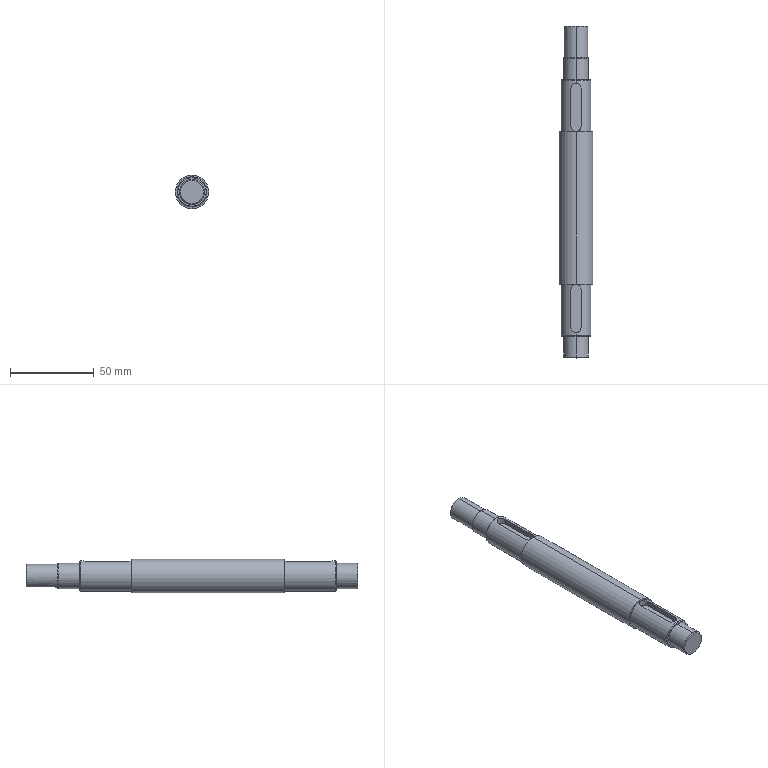Part | STEP file | 1 solid | 42 faces | box 20 x 198 x 20 mm | volume 50387 mm3 | cylinder 17 | plane 16 | cone 9 | commonest cylinder face diameters 6 x4 15 x4 18 x4 14 x2 20 x2 5 x1